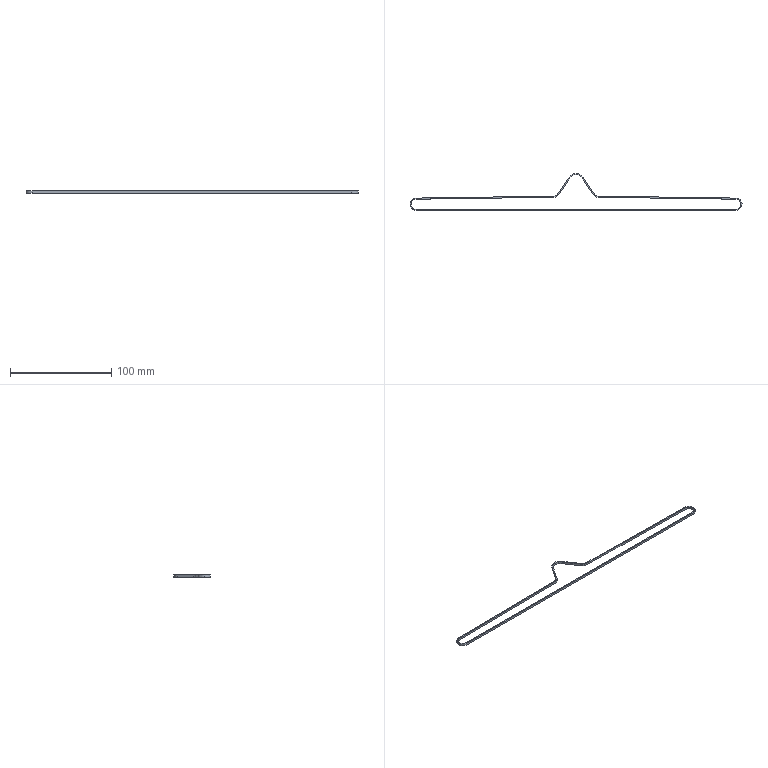Part | NX | features BREP 1 | 1 solid | 24 faces | box 328.201 x 36.406 x 2 mm | volume 1528 mm3 | plane 12 | cylinder 12 | commonest cylinder face diameters 9.981 x3 12.201 x3 10 x2 12.22 x2 14.39 x1 16.61 x1
STEP:
#1=CARTESIAN_POINT('',(-158.,-26.991,-1.));
#2=VERTEX_POINT('',#1);
#3=CARTESIAN_POINT('',(-158.,-26.991,1.));
#4=VERTEX_POINT('',#3);
#5=CARTESIAN_POINT('',(-158.,-26.991,-9.));
#6=DIRECTION('',(0.,0.,1.));
#7=VECTOR('',#6,1000.);
#8=LINE('',#5,#7);
#9=EDGE_CURVE('',#2,#4,#8,.T.);
#10=ORIENTED_EDGE('',*,*,#9,.T.);
#11=CARTESIAN_POINT('',(158.,-26.991,1.));
#12=VERTEX_POINT('',#11);
#13=CARTESIAN_POINT('',(-158.,-26.991,1.));
#14=DIRECTION('',(1.,0.,0.));
#15=VECTOR('',#14,1000.);
#16=LINE('',#13,#15);
#17=EDGE_CURVE('',#4,#12,#16,.T.);
#18=ORIENTED_EDGE('',*,*,#17,.T.);
#19=CARTESIAN_POINT('',(158.,-26.991,-1.));
#20=VERTEX_POINT('',#19);
#21=CARTESIAN_POINT('',(158.,-26.991,-9.));
#22=DIRECTION('',(0.,0.,1.));
#23=VECTOR('',#22,1000.);
#24=LINE('',#21,#23);
#25=EDGE_CURVE('',#20,#12,#24,.T.);
#26=ORIENTED_EDGE('',*,*,#25,.F.);
#27=CARTESIAN_POINT('',(158.,-26.991,-1.));
#28=DIRECTION('',(1.,0.,0.));
#29=VECTOR('',#28,1000.);
#30=LINE('',#27,#29);
#31=EDGE_CURVE('',#2,#20,#30,.T.);
#32=ORIENTED_EDGE('',*,*,#31,.F.);
#33=EDGE_LOOP('',(#10,#18,#26,#32));
#34=FACE_BOUND('',#33,.T.);
#35=CARTESIAN_POINT('',(-158.,-26.991,-9.));
#36=DIRECTION('',(0.,-1.,0.));
#37=DIRECTION('',(1.,0.,0.));
#38=AXIS2_PLACEMENT_3D('',#35,#36,#37);
#39=PLANE('',#38);
#40=ADVANCED_FACE('',(#34),#39,.F.);
#41=CARTESIAN_POINT('',(162.991,-22.,-1.));
#42=VERTEX_POINT('',#41);
#43=CARTESIAN_POINT('',(162.991,-22.,1.));
#44=VERTEX_POINT('',#43);
#45=CARTESIAN_POINT('',(162.991,-22.,-9.));
#46=DIRECTION('',(0.,0.,1.));
#47=VECTOR('',#46,1000.);
#48=LINE('',#45,#47);
#49=EDGE_CURVE('',#42,#44,#48,.T.);
#50=ORIENTED_EDGE('',*,*,#49,.F.);
#51=CARTESIAN_POINT('',(158.,-22.,-1.));
#52=DIRECTION('',(0.,0.,1.));
#53=DIRECTION('',(1.,0.,0.));
#54=AXIS2_PLACEMENT_3D('',#51,#52,#53);
#55=CIRCLE('',#54,4.991);
#56=EDGE_CURVE('',#20,#42,#55,.T.);
#57=ORIENTED_EDGE('',*,*,#56,.F.);
#58=ORIENTED_EDGE('',*,*,#25,.T.);
#59=CARTESIAN_POINT('',(158.,-22.,1.));
#60=DIRECTION('',(0.,0.,1.));
#61=DIRECTION('',(1.,0.,0.));
#62=AXIS2_PLACEMENT_3D('',#59,#60,#61);
#63=CIRCLE('',#62,4.991);
#64=EDGE_CURVE('',#12,#44,#63,.T.);
#65=ORIENTED_EDGE('',*,*,#64,.T.);
#66=EDGE_LOOP('',(#50,#57,#58,#65));
#67=FACE_BOUND('',#66,.T.);
#68=CARTESIAN_POINT('',(158.,-22.,-9.));
#69=DIRECTION('',(0.,0.,1.));
#70=DIRECTION('',(1.,0.,0.));
#71=AXIS2_PLACEMENT_3D('',#68,#69,#70);
#72=CYLINDRICAL_SURFACE('',#71,4.991);
#73=ADVANCED_FACE('',(#67),#72,.F.);
#74=CARTESIAN_POINT('',(158.07,-17.01,-1.));
#75=VERTEX_POINT('',#74);
#76=CARTESIAN_POINT('',(158.07,-17.01,1.));
#77=VERTEX_POINT('',#76);
#78=CARTESIAN_POINT('',(158.07,-17.01,-9.));
#79=DIRECTION('',(0.,0.,1.));
#80=VECTOR('',#79,1000.);
#81=LINE('',#78,#80);
#82=EDGE_CURVE('',#75,#77,#81,.T.);
#83=ORIENTED_EDGE('',*,*,#82,.T.);
#84=CARTESIAN_POINT('',(21.915,-15.109,1.));
#85=VERTEX_POINT('',#84);
#86=CARTESIAN_POINT('',(158.07,-17.01,1.));
#87=DIRECTION('',(-0.9999,0.01396,0.));
#88=VECTOR('',#87,1000.);
#89=LINE('',#86,#88);
#90=EDGE_CURVE('',#77,#85,#89,.T.);
#91=ORIENTED_EDGE('',*,*,#90,.T.);
#92=CARTESIAN_POINT('',(21.915,-15.109,-1.));
#93=VERTEX_POINT('',#92);
#94=CARTESIAN_POINT('',(21.915,-15.109,-9.));
#95=DIRECTION('',(0.,0.,1.));
#96=VECTOR('',#95,1000.);
#97=LINE('',#94,#96);
#98=EDGE_CURVE('',#93,#85,#97,.T.);
#99=ORIENTED_EDGE('',*,*,#98,.F.);
#100=CARTESIAN_POINT('',(158.07,-17.01,-1.));
#101=DIRECTION('',(-0.9999,0.01396,0.));
#102=VECTOR('',#101,1000.);
#103=LINE('',#100,#102);
#104=EDGE_CURVE('',#75,#93,#103,.T.);
#105=ORIENTED_EDGE('',*,*,#104,.F.);
#106=EDGE_LOOP('',(#83,#91,#99,#105));
#107=FACE_BOUND('',#106,.T.);
#108=CARTESIAN_POINT('',(158.07,-17.01,-9.));
#109=DIRECTION('',(0.01396,0.9999,0.));
#110=DIRECTION('',(-0.9999,0.01396,0.));
#111=AXIS2_PLACEMENT_3D('',#108,#109,#110);
#112=PLANE('',#111);
#113=ADVANCED_FACE('',(#107),#112,.F.);
#114=ORIENTED_EDGE('',*,*,#98,.T.);
#115=CARTESIAN_POINT('',(16.918,-12.391,1.));
#116=VERTEX_POINT('',#115);
#117=CARTESIAN_POINT('',(22.,-9.,1.));
#118=DIRECTION('',(0.,0.,-1.));
#119=DIRECTION('',(1.,0.,0.));
#120=AXIS2_PLACEMENT_3D('',#117,#118,#119);
#121=CIRCLE('',#120,6.11);
#122=EDGE_CURVE('',#85,#116,#121,.T.);
#123=ORIENTED_EDGE('',*,*,#122,.T.);
#124=CARTESIAN_POINT('',(16.918,-12.391,-1.));
#125=VERTEX_POINT('',#124);
#126=CARTESIAN_POINT('',(16.918,-12.391,-9.));
#127=DIRECTION('',(0.,0.,1.));
#128=VECTOR('',#127,1000.);
#129=LINE('',#126,#128);
#130=EDGE_CURVE('',#125,#116,#129,.T.);
#131=ORIENTED_EDGE('',*,*,#130,.F.);
#132=CARTESIAN_POINT('',(22.,-9.,-1.));
#133=DIRECTION('',(0.,0.,-1.));
#134=DIRECTION('',(1.,0.,0.));
#135=AXIS2_PLACEMENT_3D('',#132,#133,#134);
#136=CIRCLE('',#135,6.11);
#137=EDGE_CURVE('',#93,#125,#136,.T.);
#138=ORIENTED_EDGE('',*,*,#137,.F.);
#139=EDGE_LOOP('',(#114,#123,#131,#138));
#140=FACE_BOUND('',#139,.T.);
#141=CARTESIAN_POINT('',(22.,-9.,-9.));
#142=DIRECTION('',(0.,0.,1.));
#143=DIRECTION('',(1.,0.,0.));
#144=AXIS2_PLACEMENT_3D('',#141,#142,#143);
#145=CYLINDRICAL_SURFACE('',#144,6.11);
#146=ADVANCED_FACE('',(#140),#145,.T.);
#147=ORIENTED_EDGE('',*,*,#130,.T.);
#148=CARTESIAN_POINT('',(5.985,3.993,1.));
#149=VERTEX_POINT('',#148);
#150=CARTESIAN_POINT('',(16.918,-12.391,1.));
#151=DIRECTION('',(-0.555,0.8318,0.));
#152=VECTOR('',#151,1000.);
#153=LINE('',#150,#152);
#154=EDGE_CURVE('',#116,#149,#153,.T.);
#155=ORIENTED_EDGE('',*,*,#154,.T.);
#156=CARTESIAN_POINT('',(5.985,3.993,-1.));
#157=VERTEX_POINT('',#156);
#158=CARTESIAN_POINT('',(5.985,3.993,-9.));
#159=DIRECTION('',(0.,0.,1.));
#160=VECTOR('',#159,1000.);
#161=LINE('',#158,#160);
#162=EDGE_CURVE('',#157,#149,#161,.T.);
#163=ORIENTED_EDGE('',*,*,#162,.F.);
#164=CARTESIAN_POINT('',(64.815,-84.176,-1.));
#165=DIRECTION('',(-0.555,0.8318,0.));
#166=VECTOR('',#165,1000.);
#167=LINE('',#164,#166);
#168=EDGE_CURVE('',#125,#157,#167,.T.);
#169=ORIENTED_EDGE('',*,*,#168,.F.);
#170=EDGE_LOOP('',(#147,#155,#163,#169));
#171=FACE_BOUND('',#170,.T.);
#172=CARTESIAN_POINT('',(16.918,-12.391,-9.));
#173=DIRECTION('',(0.8318,0.555,0.));
#174=DIRECTION('',(-0.555,0.8318,0.));
#175=AXIS2_PLACEMENT_3D('',#172,#173,#174);
#176=PLANE('',#175);
#177=ADVANCED_FACE('',(#171),#176,.F.);
#178=ORIENTED_EDGE('',*,*,#162,.T.);
#179=CARTESIAN_POINT('',(-5.985,3.993,1.));
#180=VERTEX_POINT('',#179);
#181=CARTESIAN_POINT('',(0.,0.,1.));
#182=DIRECTION('',(0.,0.,1.));
#183=DIRECTION('',(1.,0.,0.));
#184=AXIS2_PLACEMENT_3D('',#181,#182,#183);
#185=CIRCLE('',#184,7.195);
#186=EDGE_CURVE('',#149,#180,#185,.T.);
#187=ORIENTED_EDGE('',*,*,#186,.T.);
#188=CARTESIAN_POINT('',(-5.985,3.993,-1.));
#189=VERTEX_POINT('',#188);
#190=CARTESIAN_POINT('',(-5.985,3.993,-9.));
#191=DIRECTION('',(0.,0.,1.));
#192=VECTOR('',#191,1000.);
#193=LINE('',#190,#192);
#194=EDGE_CURVE('',#189,#180,#193,.T.);
#195=ORIENTED_EDGE('',*,*,#194,.F.);
#196=CARTESIAN_POINT('',(0.,0.,-1.));
#197=DIRECTION('',(0.,0.,1.));
#198=DIRECTION('',(1.,0.,0.));
#199=AXIS2_PLACEMENT_3D('',#196,#197,#198);
#200=CIRCLE('',#199,7.195);
#201=EDGE_CURVE('',#157,#189,#200,.T.);
#202=ORIENTED_EDGE('',*,*,#201,.F.);
#203=EDGE_LOOP('',(#178,#187,#195,#202));
#204=FACE_BOUND('',#203,.T.);
#205=CARTESIAN_POINT('',(0.,0.,-9.));
#206=DIRECTION('',(0.,0.,1.));
#207=DIRECTION('',(1.,0.,0.));
#208=AXIS2_PLACEMENT_3D('',#205,#206,#207);
#209=CYLINDRICAL_SURFACE('',#208,7.195);
#210=ADVANCED_FACE('',(#204),#209,.F.);
#211=ORIENTED_EDGE('',*,*,#194,.T.);
#212=CARTESIAN_POINT('',(-16.918,-12.391,1.));
#213=VERTEX_POINT('',#212);
#214=CARTESIAN_POINT('',(-5.985,3.993,1.));
#215=DIRECTION('',(-0.555,-0.8318,0.));
#216=VECTOR('',#215,1000.);
#217=LINE('',#214,#216);
#218=EDGE_CURVE('',#180,#213,#217,.T.);
#219=ORIENTED_EDGE('',*,*,#218,.T.);
#220=CARTESIAN_POINT('',(-16.918,-12.391,-1.));
#221=VERTEX_POINT('',#220);
#222=CARTESIAN_POINT('',(-16.918,-12.391,-9.));
#223=DIRECTION('',(0.,0.,1.));
#224=VECTOR('',#223,1000.);
#225=LINE('',#222,#224);
#226=EDGE_CURVE('',#221,#213,#225,.T.);
#227=ORIENTED_EDGE('',*,*,#226,.F.);
#228=CARTESIAN_POINT('',(32.531,61.718,-1.));
#229=DIRECTION('',(-0.555,-0.8318,0.));
#230=VECTOR('',#229,1000.);
#231=LINE('',#228,#230);
#232=EDGE_CURVE('',#189,#221,#231,.T.);
#233=ORIENTED_EDGE('',*,*,#232,.F.);
#234=EDGE_LOOP('',(#211,#219,#227,#233));
#235=FACE_BOUND('',#234,.T.);
#236=CARTESIAN_POINT('',(-5.985,3.993,-9.));
#237=DIRECTION('',(-0.8318,0.555,0.));
#238=DIRECTION('',(-0.555,-0.8318,0.));
#239=AXIS2_PLACEMENT_3D('',#236,#237,#238);
#240=PLANE('',#239);
#241=ADVANCED_FACE('',(#235),#240,.F.);
#242=ORIENTED_EDGE('',*,*,#226,.T.);
#243=CARTESIAN_POINT('',(-21.915,-15.109,1.));
#244=VERTEX_POINT('',#243);
#245=CARTESIAN_POINT('',(-22.,-9.,1.));
#246=DIRECTION('',(0.,0.,-1.));
#247=DIRECTION('',(1.,0.,0.));
#248=AXIS2_PLACEMENT_3D('',#245,#246,#247);
#249=CIRCLE('',#248,6.11);
#250=EDGE_CURVE('',#213,#244,#249,.T.);
#251=ORIENTED_EDGE('',*,*,#250,.T.);
#252=CARTESIAN_POINT('',(-21.915,-15.109,-1.));
#253=VERTEX_POINT('',#252);
#254=CARTESIAN_POINT('',(-21.915,-15.109,-9.));
#255=DIRECTION('',(0.,0.,1.));
#256=VECTOR('',#255,1000.);
#257=LINE('',#254,#256);
#258=EDGE_CURVE('',#253,#244,#257,.T.);
#259=ORIENTED_EDGE('',*,*,#258,.F.);
#260=CARTESIAN_POINT('',(-22.,-9.,-1.));
#261=DIRECTION('',(0.,0.,-1.));
#262=DIRECTION('',(1.,0.,0.));
#263=AXIS2_PLACEMENT_3D('',#260,#261,#262);
#264=CIRCLE('',#263,6.11);
#265=EDGE_CURVE('',#221,#253,#264,.T.);
#266=ORIENTED_EDGE('',*,*,#265,.F.);
#267=EDGE_LOOP('',(#242,#251,#259,#266));
#268=FACE_BOUND('',#267,.T.);
#269=CARTESIAN_POINT('',(-22.,-9.,-9.));
#270=DIRECTION('',(0.,0.,1.));
#271=DIRECTION('',(1.,0.,0.));
#272=AXIS2_PLACEMENT_3D('',#269,#270,#271);
#273=CYLINDRICAL_SURFACE('',#272,6.11);
#274=ADVANCED_FACE('',(#268),#273,.T.);
#275=ORIENTED_EDGE('',*,*,#258,.T.);
#276=CARTESIAN_POINT('',(-158.07,-17.01,1.));
#277=VERTEX_POINT('',#276);
#278=CARTESIAN_POINT('',(-21.915,-15.109,1.));
#279=DIRECTION('',(-0.9999,-0.01396,0.));
#280=VECTOR('',#279,1000.);
#281=LINE('',#278,#280);
#282=EDGE_CURVE('',#244,#277,#281,.T.);
#283=ORIENTED_EDGE('',*,*,#282,.T.);
#284=CARTESIAN_POINT('',(-158.07,-17.01,-1.));
#285=VERTEX_POINT('',#284);
#286=CARTESIAN_POINT('',(-158.07,-17.01,-9.));
#287=DIRECTION('',(0.,0.,1.));
#288=VECTOR('',#287,1000.);
#289=LINE('',#286,#288);
#290=EDGE_CURVE('',#285,#277,#289,.T.);
#291=ORIENTED_EDGE('',*,*,#290,.F.);
#292=CARTESIAN_POINT('',(157.869,-12.6,-1.));
#293=DIRECTION('',(-0.9999,-0.01396,0.));
#294=VECTOR('',#293,1000.);
#295=LINE('',#292,#294);
#296=EDGE_CURVE('',#253,#285,#295,.T.);
#297=ORIENTED_EDGE('',*,*,#296,.F.);
#298=EDGE_LOOP('',(#275,#283,#291,#297));
#299=FACE_BOUND('',#298,.T.);
#300=CARTESIAN_POINT('',(-21.915,-15.109,-9.));
#301=DIRECTION('',(-0.01396,0.9999,0.));
#302=DIRECTION('',(-0.9999,-0.01396,0.));
#303=AXIS2_PLACEMENT_3D('',#300,#301,#302);
#304=PLANE('',#303);
#305=ADVANCED_FACE('',(#299),#304,.F.);
#306=ORIENTED_EDGE('',*,*,#290,.T.);
#307=CARTESIAN_POINT('',(-158.,-22.,1.));
#308=DIRECTION('',(0.,0.,1.));
#309=DIRECTION('',(1.,0.,0.));
#310=AXIS2_PLACEMENT_3D('',#307,#308,#309);
#311=CIRCLE('',#310,4.991);
#312=EDGE_CURVE('',#277,#4,#311,.T.);
#313=ORIENTED_EDGE('',*,*,#312,.T.);
#314=ORIENTED_EDGE('',*,*,#9,.F.);
#315=CARTESIAN_POINT('',(-158.,-22.,-1.));
#316=DIRECTION('',(0.,0.,1.));
#317=DIRECTION('',(1.,0.,0.));
#318=AXIS2_PLACEMENT_3D('',#315,#316,#317);
#319=CIRCLE('',#318,4.991);
#320=EDGE_CURVE('',#285,#2,#319,.T.);
#321=ORIENTED_EDGE('',*,*,#320,.F.);
#322=EDGE_LOOP('',(#306,#313,#314,#321));
#323=FACE_BOUND('',#322,.T.);
#324=CARTESIAN_POINT('',(-158.,-22.,-9.));
#325=DIRECTION('',(0.,0.,1.));
#326=DIRECTION('',(1.,0.,0.));
#327=AXIS2_PLACEMENT_3D('',#324,#325,#326);
#328=CYLINDRICAL_SURFACE('',#327,4.991);
#329=ADVANCED_FACE('',(#323),#328,.F.);
#330=CARTESIAN_POINT('',(158.,-28.101,-1.));
#331=VERTEX_POINT('',#330);
#332=CARTESIAN_POINT('',(158.085,-15.9,-1.));
#333=VERTEX_POINT('',#332);
#334=CARTESIAN_POINT('',(158.,-22.,-1.));
#335=DIRECTION('',(0.,0.,1.));
#336=DIRECTION('',(1.,0.,0.));
#337=AXIS2_PLACEMENT_3D('',#334,#335,#336);
#338=CIRCLE('',#337,6.101);
#339=EDGE_CURVE('',#331,#333,#338,.T.);
#340=ORIENTED_EDGE('',*,*,#339,.F.);
#341=CARTESIAN_POINT('',(-158.,-28.101,-1.));
#342=VERTEX_POINT('',#341);
#343=CARTESIAN_POINT('',(158.,-28.101,-1.));
#344=DIRECTION('',(1.,0.,0.));
#345=VECTOR('',#344,1000.);
#346=LINE('',#343,#345);
#347=EDGE_CURVE('',#342,#331,#346,.T.);
#348=ORIENTED_EDGE('',*,*,#347,.F.);
#349=CARTESIAN_POINT('',(-164.101,-22.,-1.));
#350=VERTEX_POINT('',#349);
#351=CARTESIAN_POINT('',(-158.,-22.,-1.));
#352=DIRECTION('',(0.,0.,1.));
#353=DIRECTION('',(-1.,0.,0.));
#354=AXIS2_PLACEMENT_3D('',#351,#352,#353);
#355=CIRCLE('',#354,6.101);
#356=EDGE_CURVE('',#350,#342,#355,.T.);
#357=ORIENTED_EDGE('',*,*,#356,.F.);
#358=CARTESIAN_POINT('',(-158.085,-15.9,-1.));
#359=VERTEX_POINT('',#358);
#360=CARTESIAN_POINT('',(-158.,-22.,-1.));
#361=DIRECTION('',(0.,0.,1.));
#362=DIRECTION('',(-1.,0.,0.));
#363=AXIS2_PLACEMENT_3D('',#360,#361,#362);
#364=CIRCLE('',#363,6.101);
#365=EDGE_CURVE('',#359,#350,#364,.T.);
#366=ORIENTED_EDGE('',*,*,#365,.F.);
#367=CARTESIAN_POINT('',(-21.93,-14.,-1.));
#368=VERTEX_POINT('',#367);
#369=CARTESIAN_POINT('',(-21.93,-14.,-1.));
#370=DIRECTION('',(-0.9999,-0.01396,0.));
#371=VECTOR('',#370,1000.);
#372=LINE('',#369,#371);
#373=EDGE_CURVE('',#368,#359,#372,.T.);
#374=ORIENTED_EDGE('',*,*,#373,.F.);
#375=CARTESIAN_POINT('',(-17.841,-11.775,-1.));
#376=VERTEX_POINT('',#375);
#377=CARTESIAN_POINT('',(-22.,-9.,-1.));
#378=DIRECTION('',(0.,0.,-1.));
#379=DIRECTION('',(-1.,0.,0.));
#380=AXIS2_PLACEMENT_3D('',#377,#378,#379);
#381=CIRCLE('',#380,5.);
#382=EDGE_CURVE('',#376,#368,#381,.T.);
#383=ORIENTED_EDGE('',*,*,#382,.F.);
#384=CARTESIAN_POINT('',(-6.908,4.61,-1.));
#385=VERTEX_POINT('',#384);
#386=CARTESIAN_POINT('',(-17.841,-11.775,-1.));
#387=DIRECTION('',(-0.555,-0.8318,0.));
#388=VECTOR('',#387,1000.);
#389=LINE('',#386,#388);
#390=EDGE_CURVE('',#385,#376,#389,.T.);
#391=ORIENTED_EDGE('',*,*,#390,.F.);
#392=CARTESIAN_POINT('',(6.908,4.61,-1.));
#393=VERTEX_POINT('',#392);
#394=CARTESIAN_POINT('',(0.,0.,-1.));
#395=DIRECTION('',(0.,0.,1.));
#396=DIRECTION('',(1.,0.,0.));
#397=AXIS2_PLACEMENT_3D('',#394,#395,#396);
#398=CIRCLE('',#397,8.305);
#399=EDGE_CURVE('',#393,#385,#398,.T.);
#400=ORIENTED_EDGE('',*,*,#399,.F.);
#401=CARTESIAN_POINT('',(17.841,-11.775,-1.));
#402=VERTEX_POINT('',#401);
#403=CARTESIAN_POINT('',(17.841,-11.775,-1.));
#404=DIRECTION('',(-0.555,0.8318,0.));
#405=VECTOR('',#404,1000.);
#406=LINE('',#403,#405);
#407=EDGE_CURVE('',#402,#393,#406,.T.);
#408=ORIENTED_EDGE('',*,*,#407,.F.);
#409=CARTESIAN_POINT('',(21.93,-14.,-1.));
#410=VERTEX_POINT('',#409);
#411=CARTESIAN_POINT('',(22.,-9.,-1.));
#412=DIRECTION('',(0.,0.,-1.));
#413=DIRECTION('',(1.,0.,0.));
#414=AXIS2_PLACEMENT_3D('',#411,#412,#413);
#415=CIRCLE('',#414,5.);
#416=EDGE_CURVE('',#410,#402,#415,.T.);
#417=ORIENTED_EDGE('',*,*,#416,.F.);
#418=CARTESIAN_POINT('',(21.93,-14.,-1.));
#419=DIRECTION('',(-0.9999,0.01396,0.));
#420=VECTOR('',#419,1000.);
#421=LINE('',#418,#420);
#422=EDGE_CURVE('',#333,#410,#421,.T.);
#423=ORIENTED_EDGE('',*,*,#422,.F.);
#424=EDGE_LOOP('',(#340,#348,#357,#366,#374,#383,#391,#400,#408,#417,#423));
#425=FACE_BOUND('',#424,.T.);
#426=ORIENTED_EDGE('',*,*,#296,.T.);
#427=ORIENTED_EDGE('',*,*,#320,.T.);
#428=ORIENTED_EDGE('',*,*,#31,.T.);
#429=ORIENTED_EDGE('',*,*,#56,.T.);
#430=CARTESIAN_POINT('',(158.,-22.,-1.));
#431=DIRECTION('',(0.,0.,1.));
#432=DIRECTION('',(1.,0.,0.));
#433=AXIS2_PLACEMENT_3D('',#430,#431,#432);
#434=CIRCLE('',#433,4.991);
#435=EDGE_CURVE('',#42,#75,#434,.T.);
#436=ORIENTED_EDGE('',*,*,#435,.T.);
#437=ORIENTED_EDGE('',*,*,#104,.T.);
#438=ORIENTED_EDGE('',*,*,#137,.T.);
#439=ORIENTED_EDGE('',*,*,#168,.T.);
#440=ORIENTED_EDGE('',*,*,#201,.T.);
#441=ORIENTED_EDGE('',*,*,#232,.T.);
#442=ORIENTED_EDGE('',*,*,#265,.T.);
#443=EDGE_LOOP('',(#426,#427,#428,#429,#436,#437,#438,#439,#440,#441,#442));
#444=FACE_BOUND('',#443,.T.);
#445=CARTESIAN_POINT('',(158.,-22.,-1.));
#446=DIRECTION('',(0.,0.,1.));
#447=DIRECTION('',(1.,0.,0.));
#448=AXIS2_PLACEMENT_3D('',#445,#446,#447);
#449=PLANE('',#448);
#450=ADVANCED_FACE('',(#425,#444),#449,.F.);
#451=CARTESIAN_POINT('',(158.,-28.101,1.));
#452=VERTEX_POINT('',#451);
#453=CARTESIAN_POINT('',(158.085,-15.9,1.));
#454=VERTEX_POINT('',#453);
#455=CARTESIAN_POINT('',(158.,-22.,1.));
#456=DIRECTION('',(0.,0.,1.));
#457=DIRECTION('',(1.,0.,0.));
#458=AXIS2_PLACEMENT_3D('',#455,#456,#457);
#459=CIRCLE('',#458,6.101);
#460=EDGE_CURVE('',#452,#454,#459,.T.);
#461=ORIENTED_EDGE('',*,*,#460,.T.);
#462=CARTESIAN_POINT('',(21.93,-14.,1.));
#463=VERTEX_POINT('',#462);
#464=CARTESIAN_POINT('',(21.93,-14.,1.));
#465=DIRECTION('',(-0.9999,0.01396,0.));
#466=VECTOR('',#465,1000.);
#467=LINE('',#464,#466);
#468=EDGE_CURVE('',#454,#463,#467,.T.);
#469=ORIENTED_EDGE('',*,*,#468,.T.);
#470=CARTESIAN_POINT('',(17.841,-11.775,1.));
#471=VERTEX_POINT('',#470);
#472=CARTESIAN_POINT('',(22.,-9.,1.));
#473=DIRECTION('',(0.,0.,-1.));
#474=DIRECTION('',(1.,0.,0.));
#475=AXIS2_PLACEMENT_3D('',#472,#473,#474);
#476=CIRCLE('',#475,5.);
#477=EDGE_CURVE('',#463,#471,#476,.T.);
#478=ORIENTED_EDGE('',*,*,#477,.T.);
#479=CARTESIAN_POINT('',(6.908,4.61,1.));
#480=VERTEX_POINT('',#479);
#481=CARTESIAN_POINT('',(17.841,-11.775,1.));
#482=DIRECTION('',(-0.555,0.8318,0.));
#483=VECTOR('',#482,1000.);
#484=LINE('',#481,#483);
#485=EDGE_CURVE('',#471,#480,#484,.T.);
#486=ORIENTED_EDGE('',*,*,#485,.T.);
#487=CARTESIAN_POINT('',(-6.908,4.61,1.));
#488=VERTEX_POINT('',#487);
#489=CARTESIAN_POINT('',(0.,0.,1.));
#490=DIRECTION('',(0.,0.,1.));
#491=DIRECTION('',(1.,0.,0.));
#492=AXIS2_PLACEMENT_3D('',#489,#490,#491);
#493=CIRCLE('',#492,8.305);
#494=EDGE_CURVE('',#480,#488,#493,.T.);
#495=ORIENTED_EDGE('',*,*,#494,.T.);
#496=CARTESIAN_POINT('',(-17.841,-11.775,1.));
#497=VERTEX_POINT('',#496);
#498=CARTESIAN_POINT('',(-17.841,-11.775,1.));
#499=DIRECTION('',(-0.555,-0.8318,0.));
#500=VECTOR('',#499,1000.);
#501=LINE('',#498,#500);
#502=EDGE_CURVE('',#488,#497,#501,.T.);
#503=ORIENTED_EDGE('',*,*,#502,.T.);
#504=CARTESIAN_POINT('',(-21.93,-14.,1.));
#505=VERTEX_POINT('',#504);
#506=CARTESIAN_POINT('',(-22.,-9.,1.));
#507=DIRECTION('',(0.,0.,-1.));
#508=DIRECTION('',(-1.,0.,0.));
#509=AXIS2_PLACEMENT_3D('',#506,#507,#508);
#510=CIRCLE('',#509,5.);
#511=EDGE_CURVE('',#497,#505,#510,.T.);
#512=ORIENTED_EDGE('',*,*,#511,.T.);
#513=CARTESIAN_POINT('',(-158.085,-15.9,1.));
#514=VERTEX_POINT('',#513);
#515=CARTESIAN_POINT('',(-21.93,-14.,1.));
#516=DIRECTION('',(-0.9999,-0.01396,0.));
#517=VECTOR('',#516,1000.);
#518=LINE('',#515,#517);
#519=EDGE_CURVE('',#505,#514,#518,.T.);
#520=ORIENTED_EDGE('',*,*,#519,.T.);
#521=CARTESIAN_POINT('',(-164.101,-22.,1.));
#522=VERTEX_POINT('',#521);
#523=CARTESIAN_POINT('',(-158.,-22.,1.));
#524=DIRECTION('',(0.,0.,1.));
#525=DIRECTION('',(-1.,0.,0.));
#526=AXIS2_PLACEMENT_3D('',#523,#524,#525);
#527=CIRCLE('',#526,6.101);
#528=EDGE_CURVE('',#514,#522,#527,.T.);
#529=ORIENTED_EDGE('',*,*,#528,.T.);
#530=CARTESIAN_POINT('',(-158.,-28.101,1.));
#531=VERTEX_POINT('',#530);
#532=CARTESIAN_POINT('',(-158.,-22.,1.));
#533=DIRECTION('',(0.,0.,1.));
#534=DIRECTION('',(-1.,0.,0.));
#535=AXIS2_PLACEMENT_3D('',#532,#533,#534);
#536=CIRCLE('',#535,6.101);
#537=EDGE_CURVE('',#522,#531,#536,.T.);
#538=ORIENTED_EDGE('',*,*,#537,.T.);
#539=CARTESIAN_POINT('',(158.,-28.101,1.));
#540=DIRECTION('',(1.,0.,0.));
#541=VECTOR('',#540,1000.);
#542=LINE('',#539,#541);
#543=EDGE_CURVE('',#531,#452,#542,.T.);
#544=ORIENTED_EDGE('',*,*,#543,.T.);
#545=EDGE_LOOP('',(#461,#469,#478,#486,#495,#503,#512,#520,#529,#538,#544));
#546=FACE_BOUND('',#545,.T.);
#547=ORIENTED_EDGE('',*,*,#312,.F.);
#548=ORIENTED_EDGE('',*,*,#282,.F.);
#549=ORIENTED_EDGE('',*,*,#250,.F.);
#550=ORIENTED_EDGE('',*,*,#218,.F.);
#551=ORIENTED_EDGE('',*,*,#186,.F.);
#552=ORIENTED_EDGE('',*,*,#154,.F.);
#553=ORIENTED_EDGE('',*,*,#122,.F.);
#554=ORIENTED_EDGE('',*,*,#90,.F.);
#555=CARTESIAN_POINT('',(158.,-22.,1.));
#556=DIRECTION('',(0.,0.,1.));
#557=DIRECTION('',(1.,0.,0.));
#558=AXIS2_PLACEMENT_3D('',#555,#556,#557);
#559=CIRCLE('',#558,4.991);
#560=EDGE_CURVE('',#44,#77,#559,.T.);
#561=ORIENTED_EDGE('',*,*,#560,.F.);
#562=ORIENTED_EDGE('',*,*,#64,.F.);
#563=ORIENTED_EDGE('',*,*,#17,.F.);
#564=EDGE_LOOP('',(#547,#548,#549,#550,#551,#552,#553,#554,#561,#562,#563));
#565=FACE_BOUND('',#564,.T.);
#566=CARTESIAN_POINT('',(158.,-22.,1.));
#567=DIRECTION('',(0.,0.,1.));
#568=DIRECTION('',(1.,0.,0.));
#569=AXIS2_PLACEMENT_3D('',#566,#567,#568);
#570=PLANE('',#569);
#571=ADVANCED_FACE('',(#546,#565),#570,.T.);
#572=ORIENTED_EDGE('',*,*,#347,.T.);
#573=CARTESIAN_POINT('',(158.,-28.101,1.));
#574=DIRECTION('',(0.,0.,-1.));
#575=VECTOR('',#574,1000.);
#576=LINE('',#573,#575);
#577=EDGE_CURVE('',#452,#331,#576,.T.);
#578=ORIENTED_EDGE('',*,*,#577,.F.);
#579=ORIENTED_EDGE('',*,*,#543,.F.);
#580=CARTESIAN_POINT('',(-158.,-28.101,1.));
#581=DIRECTION('',(0.,0.,-1.));
#582=VECTOR('',#581,1000.);
#583=LINE('',#580,#582);
#584=EDGE_CURVE('',#531,#342,#583,.T.);
#585=ORIENTED_EDGE('',*,*,#584,.T.);
#586=EDGE_LOOP('',(#572,#578,#579,#585));
#587=FACE_BOUND('',#586,.T.);
#588=CARTESIAN_POINT('',(158.,-28.101,1.));
#589=DIRECTION('',(0.,1.,0.));
#590=DIRECTION('',(-1.,0.,0.));
#591=AXIS2_PLACEMENT_3D('',#588,#589,#590);
#592=PLANE('',#591);
#593=ADVANCED_FACE('',(#587),#592,.F.);
#594=CARTESIAN_POINT('',(-164.101,-22.,1.));
#595=DIRECTION('',(0.,0.,-1.));
#596=VECTOR('',#595,1000.);
#597=LINE('',#594,#596);
#598=EDGE_CURVE('',#522,#350,#597,.T.);
#599=ORIENTED_EDGE('',*,*,#598,.F.);
#600=ORIENTED_EDGE('',*,*,#528,.F.);
#601=CARTESIAN_POINT('',(-158.085,-15.9,1.));
#602=DIRECTION('',(0.,0.,-1.));
#603=VECTOR('',#602,1000.);
#604=LINE('',#601,#603);
#605=EDGE_CURVE('',#514,#359,#604,.T.);
#606=ORIENTED_EDGE('',*,*,#605,.T.);
#607=ORIENTED_EDGE('',*,*,#365,.T.);
#608=EDGE_LOOP('',(#599,#600,#606,#607));
#609=FACE_BOUND('',#608,.T.);
#610=CARTESIAN_POINT('',(-158.,-22.,1.));
#611=DIRECTION('',(0.,0.,-1.));
#612=DIRECTION('',(-1.,0.,0.));
#613=AXIS2_PLACEMENT_3D('',#610,#611,#612);
#614=CYLINDRICAL_SURFACE('',#613,6.101);
#615=ADVANCED_FACE('',(#609),#614,.T.);
#616=ORIENTED_EDGE('',*,*,#373,.T.);
#617=ORIENTED_EDGE('',*,*,#605,.F.);
#618=ORIENTED_EDGE('',*,*,#519,.F.);
#619=CARTESIAN_POINT('',(-21.93,-14.,1.));
#620=DIRECTION('',(0.,0.,-1.));
#621=VECTOR('',#620,1000.);
#622=LINE('',#619,#621);
#623=EDGE_CURVE('',#505,#368,#622,.T.);
#624=ORIENTED_EDGE('',*,*,#623,.T.);
#625=EDGE_LOOP('',(#616,#617,#618,#624));
#626=FACE_BOUND('',#625,.T.);
#627=CARTESIAN_POINT('',(-21.93,-14.,1.));
#628=DIRECTION('',(0.01396,-0.9999,0.));
#629=DIRECTION('',(0.9999,0.01396,0.));
#630=AXIS2_PLACEMENT_3D('',#627,#628,#629);
#631=PLANE('',#630);
#632=ADVANCED_FACE('',(#626),#631,.F.);
#633=ORIENTED_EDGE('',*,*,#382,.T.);
#634=ORIENTED_EDGE('',*,*,#623,.F.);
#635=ORIENTED_EDGE('',*,*,#511,.F.);
#636=CARTESIAN_POINT('',(-17.841,-11.775,1.));
#637=DIRECTION('',(0.,0.,-1.));
#638=VECTOR('',#637,1000.);
#639=LINE('',#636,#638);
#640=EDGE_CURVE('',#497,#376,#639,.T.);
#641=ORIENTED_EDGE('',*,*,#640,.T.);
#642=EDGE_LOOP('',(#633,#634,#635,#641));
#643=FACE_BOUND('',#642,.T.);
#644=CARTESIAN_POINT('',(-22.,-9.,1.));
#645=DIRECTION('',(0.,0.,-1.));
#646=DIRECTION('',(-1.,0.,0.));
#647=AXIS2_PLACEMENT_3D('',#644,#645,#646);
#648=CYLINDRICAL_SURFACE('',#647,5.);
#649=ADVANCED_FACE('',(#643),#648,.F.);
#650=ORIENTED_EDGE('',*,*,#390,.T.);
#651=ORIENTED_EDGE('',*,*,#640,.F.);
#652=ORIENTED_EDGE('',*,*,#502,.F.);
#653=CARTESIAN_POINT('',(-6.908,4.61,1.));
#654=DIRECTION('',(0.,0.,-1.));
#655=VECTOR('',#654,1000.);
#656=LINE('',#653,#655);
#657=EDGE_CURVE('',#488,#385,#656,.T.);
#658=ORIENTED_EDGE('',*,*,#657,.T.);
#659=EDGE_LOOP('',(#650,#651,#652,#658));
#660=FACE_BOUND('',#659,.T.);
#661=CARTESIAN_POINT('',(-17.841,-11.775,1.));
#662=DIRECTION('',(0.8318,-0.555,0.));
#663=DIRECTION('',(0.555,0.8318,0.));
#664=AXIS2_PLACEMENT_3D('',#661,#662,#663);
#665=PLANE('',#664);
#666=ADVANCED_FACE('',(#660),#665,.F.);
#667=ORIENTED_EDGE('',*,*,#399,.T.);
#668=ORIENTED_EDGE('',*,*,#657,.F.);
#669=ORIENTED_EDGE('',*,*,#494,.F.);
#670=CARTESIAN_POINT('',(6.908,4.61,1.));
#671=DIRECTION('',(0.,0.,-1.));
#672=VECTOR('',#671,1000.);
#673=LINE('',#670,#672);
#674=EDGE_CURVE('',#480,#393,#673,.T.);
#675=ORIENTED_EDGE('',*,*,#674,.T.);
#676=EDGE_LOOP('',(#667,#668,#669,#675));
#677=FACE_BOUND('',#676,.T.);
#678=CARTESIAN_POINT('',(0.,0.,1.));
#679=DIRECTION('',(0.,0.,-1.));
#680=DIRECTION('',(-1.,0.,0.));
#681=AXIS2_PLACEMENT_3D('',#678,#679,#680);
#682=CYLINDRICAL_SURFACE('',#681,8.305);
#683=ADVANCED_FACE('',(#677),#682,.T.);
#684=ORIENTED_EDGE('',*,*,#407,.T.);
#685=ORIENTED_EDGE('',*,*,#674,.F.);
#686=ORIENTED_EDGE('',*,*,#485,.F.);
#687=CARTESIAN_POINT('',(17.841,-11.775,1.));
#688=DIRECTION('',(0.,0.,-1.));
#689=VECTOR('',#688,1000.);
#690=LINE('',#687,#689);
#691=EDGE_CURVE('',#471,#402,#690,.T.);
#692=ORIENTED_EDGE('',*,*,#691,.T.);
#693=EDGE_LOOP('',(#684,#685,#686,#692));
#694=FACE_BOUND('',#693,.T.);
#695=CARTESIAN_POINT('',(17.841,-11.775,1.));
#696=DIRECTION('',(-0.8318,-0.555,0.));
#697=DIRECTION('',(0.555,-0.8318,0.));
#698=AXIS2_PLACEMENT_3D('',#695,#696,#697);
#699=PLANE('',#698);
#700=ADVANCED_FACE('',(#694),#699,.F.);
#701=ORIENTED_EDGE('',*,*,#416,.T.);
#702=ORIENTED_EDGE('',*,*,#691,.F.);
#703=ORIENTED_EDGE('',*,*,#477,.F.);
#704=CARTESIAN_POINT('',(21.93,-14.,1.));
#705=DIRECTION('',(0.,0.,-1.));
#706=VECTOR('',#705,1000.);
#707=LINE('',#704,#706);
#708=EDGE_CURVE('',#463,#410,#707,.T.);
#709=ORIENTED_EDGE('',*,*,#708,.T.);
#710=EDGE_LOOP('',(#701,#702,#703,#709));
#711=FACE_BOUND('',#710,.T.);
#712=CARTESIAN_POINT('',(22.,-9.,1.));
#713=DIRECTION('',(0.,0.,-1.));
#714=DIRECTION('',(-1.,0.,0.));
#715=AXIS2_PLACEMENT_3D('',#712,#713,#714);
#716=CYLINDRICAL_SURFACE('',#715,5.);
#717=ADVANCED_FACE('',(#711),#716,.F.);
#718=ORIENTED_EDGE('',*,*,#422,.T.);
#719=ORIENTED_EDGE('',*,*,#708,.F.);
#720=ORIENTED_EDGE('',*,*,#468,.F.);
#721=CARTESIAN_POINT('',(158.085,-15.9,1.));
#722=DIRECTION('',(0.,0.,-1.));
#723=VECTOR('',#722,1000.);
#724=LINE('',#721,#723);
#725=EDGE_CURVE('',#454,#333,#724,.T.);
#726=ORIENTED_EDGE('',*,*,#725,.T.);
#727=EDGE_LOOP('',(#718,#719,#720,#726));
#728=FACE_BOUND('',#727,.T.);
#729=CARTESIAN_POINT('',(21.93,-14.,1.));
#730=DIRECTION('',(-0.01396,-0.9999,0.));
#731=DIRECTION('',(0.9999,-0.01396,0.));
#732=AXIS2_PLACEMENT_3D('',#729,#730,#731);
#733=PLANE('',#732);
#734=ADVANCED_FACE('',(#728),#733,.F.);
#735=ORIENTED_EDGE('',*,*,#339,.T.);
#736=ORIENTED_EDGE('',*,*,#725,.F.);
#737=ORIENTED_EDGE('',*,*,#460,.F.);
#738=ORIENTED_EDGE('',*,*,#577,.T.);
#739=EDGE_LOOP('',(#735,#736,#737,#738));
#740=FACE_BOUND('',#739,.T.);
#741=CARTESIAN_POINT('',(158.,-22.,1.));
#742=DIRECTION('',(0.,0.,-1.));
#743=DIRECTION('',(-1.,0.,0.));
#744=AXIS2_PLACEMENT_3D('',#741,#742,#743);
#745=CYLINDRICAL_SURFACE('',#744,6.101);
#746=ADVANCED_FACE('',(#740),#745,.T.);
#747=ORIENTED_EDGE('',*,*,#537,.F.);
#748=ORIENTED_EDGE('',*,*,#598,.T.);
#749=ORIENTED_EDGE('',*,*,#356,.T.);
#750=ORIENTED_EDGE('',*,*,#584,.F.);
#751=EDGE_LOOP('',(#747,#748,#749,#750));
#752=FACE_BOUND('',#751,.T.);
#753=CARTESIAN_POINT('',(-158.,-22.,1.));
#754=DIRECTION('',(0.,0.,-1.));
#755=DIRECTION('',(-1.,0.,0.));
#756=AXIS2_PLACEMENT_3D('',#753,#754,#755);
#757=CYLINDRICAL_SURFACE('',#756,6.101);
#758=ADVANCED_FACE('',(#752),#757,.T.);
#759=ORIENTED_EDGE('',*,*,#435,.F.);
#760=ORIENTED_EDGE('',*,*,#49,.T.);
#761=ORIENTED_EDGE('',*,*,#560,.T.);
#762=ORIENTED_EDGE('',*,*,#82,.F.);
#763=EDGE_LOOP('',(#759,#760,#761,#762));
#764=FACE_BOUND('',#763,.T.);
#765=CARTESIAN_POINT('',(158.,-22.,-9.));
#766=DIRECTION('',(0.,0.,1.));
#767=DIRECTION('',(1.,0.,0.));
#768=AXIS2_PLACEMENT_3D('',#765,#766,#767);
#769=CYLINDRICAL_SURFACE('',#768,4.991);
#770=ADVANCED_FACE('',(#764),#769,.F.);
#771=CLOSED_SHELL('',(#40,#73,#113,#146,#177,#210,#241,#274,#305,#329,#450,#571,#593,#615,#632,#649,#666,#683,#700,#717,#734,#746,#758,#770));
#772=MANIFOLD_SOLID_BREP('',#771);
#773=(LENGTH_UNIT()NAMED_UNIT(*)SI_UNIT(.MILLI.,.METRE.));
#774=UNCERTAINTY_MEASURE_WITH_UNIT(LENGTH_MEASURE(0.00001),#773,'','');
#775=(NAMED_UNIT(*)PLANE_ANGLE_UNIT()SI_UNIT($,.RADIAN.));
#776=(NAMED_UNIT(*)SI_UNIT($,.STERADIAN.)SOLID_ANGLE_UNIT());
#777=(GEOMETRIC_REPRESENTATION_CONTEXT(3)GLOBAL_UNCERTAINTY_ASSIGNED_CONTEXT((#774))GLOBAL_UNIT_ASSIGNED_CONTEXT((#773,#775,#776))REPRESENTATION_CONTEXT('',''));
#778=ADVANCED_BREP_SHAPE_REPRESENTATION('',(#772),#777);